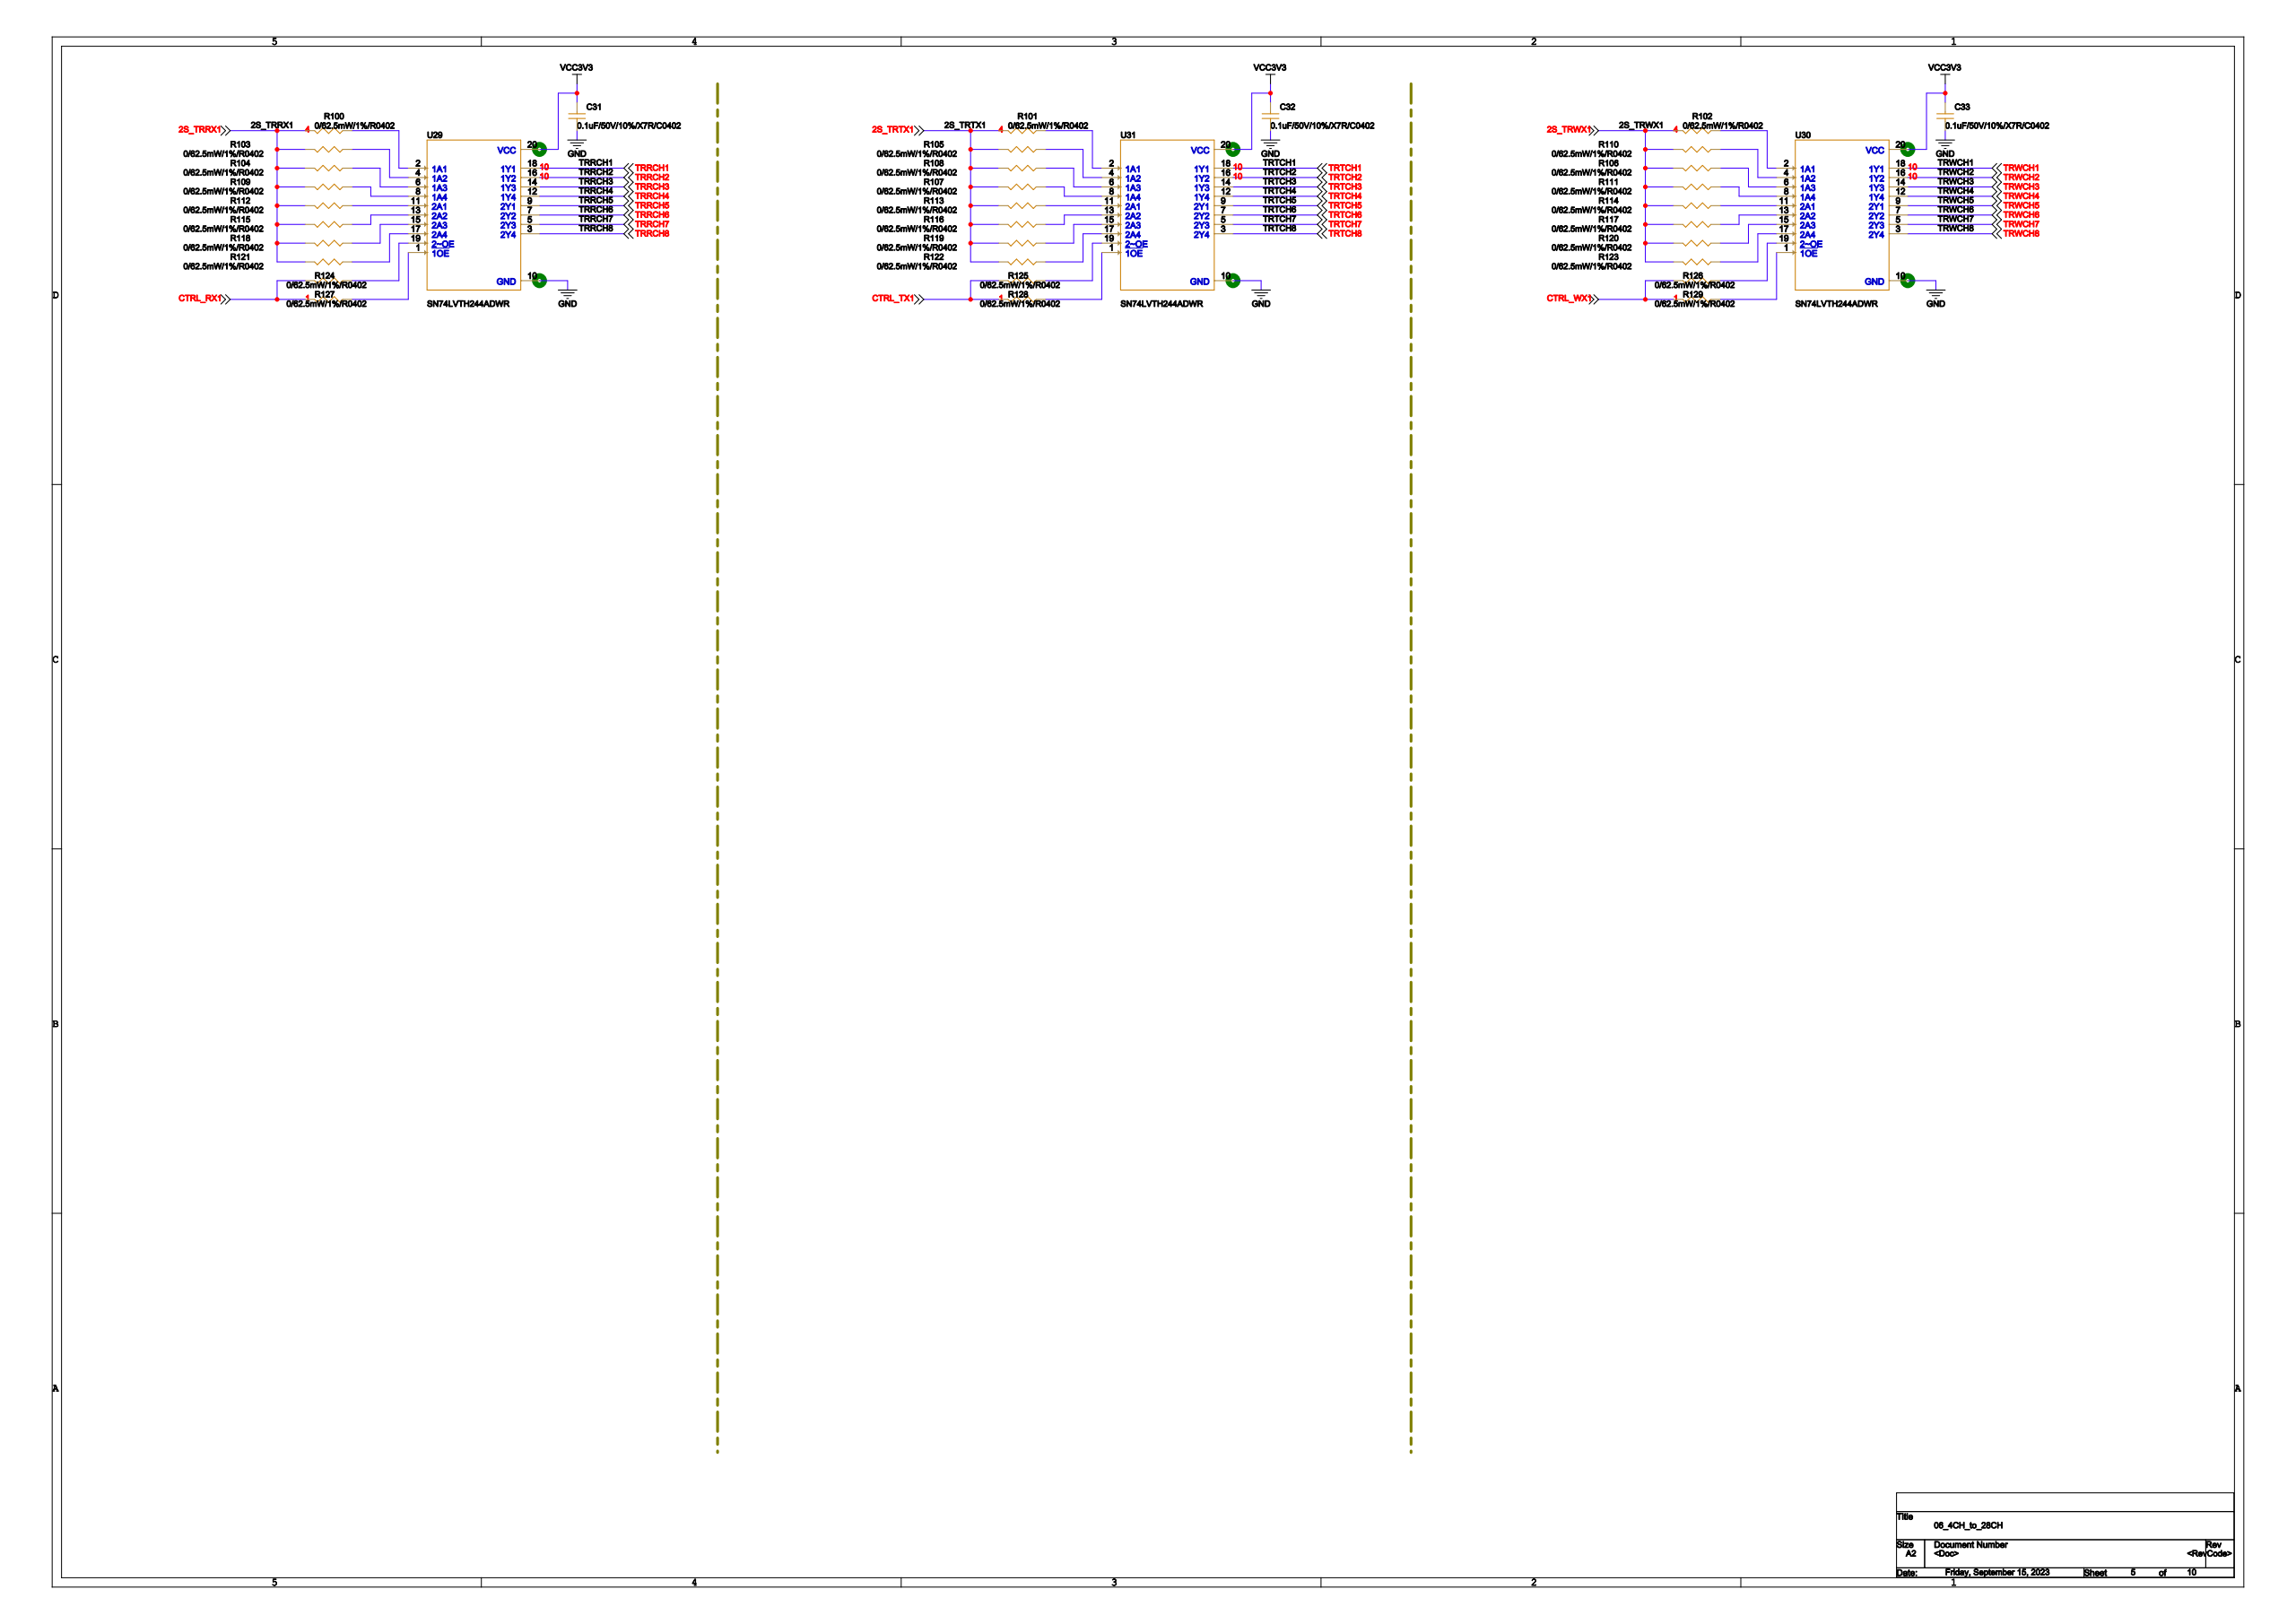Circuit board | Cadence Allegro | 634 parts | 645 nets | one sheet of the schematic
Parts on this sheet (reference | value | footprint):
C31 | 0.1uF/50V/10%/X7R/C0402 | 0402
C32 | 0.1uF/50V/10%/X7R/C0402 | 0402
C33 | 0.1uF/50V/10%/X7R/C0402 | 0402
R100 | 0/62.5mW/1%/R0402 | 0402
R101 | 0/62.5mW/1%/R0402 | 0402
R102 | 0/62.5mW/1%/R0402 | 0402
R103 | 0/62.5mW/1%/R0402 | 0402
R104 | 0/62.5mW/1%/R0402 | 0402
R105 | 0/62.5mW/1%/R0402 | 0402
R106 | 0/62.5mW/1%/R0402 | 0402
R107 | 0/62.5mW/1%/R0402 | 0402
R108 | 0/62.5mW/1%/R0402 | 0402
R109 | 0/62.5mW/1%/R0402 | 0402
R110 | 0/62.5mW/1%/R0402 | 0402
R111 | 0/62.5mW/1%/R0402 | 0402
R112 | 0/62.5mW/1%/R0402 | 0402
R113 | 0/62.5mW/1%/R0402 | 0402
R114 | 0/62.5mW/1%/R0402 | 0402
R115 | 0/62.5mW/1%/R0402 | 0402
R116 | 0/62.5mW/1%/R0402 | 0402
R117 | 0/62.5mW/1%/R0402 | 0402
R118 | 0/62.5mW/1%/R0402 | 0402
R119 | 0/62.5mW/1%/R0402 | 0402
R120 | 0/62.5mW/1%/R0402 | 0402
R121 | 0/62.5mW/1%/R0402 | 0402
R122 | 0/62.5mW/1%/R0402 | 0402
R123 | 0/62.5mW/1%/R0402 | 0402
R124 | 0/62.5mW/1%/R0402 | 0402
R125 | 0/62.5mW/1%/R0402 | 0402
R126 | 0/62.5mW/1%/R0402 | 0402
R127 | 0/62.5mW/1%/R0402 | 0402
R128 | 0/62.5mW/1%/R0402 | 0402
R129 | 0/62.5mW/1%/R0402 | 0402
U29 | SN74LVTH244ADWR | SOIC127P1030X265-20N
U30 | SN74LVTH244ADWR | SOIC127P1030X265-20N
U31 | SN74LVTH244ADWR | SOIC127P1030X265-20N
Nets of these parts (net: part-pin ...):
AGND: C31-2 C32-2 C33-2 U29-10 U30-10 U31-10
3.3V: C31-1 C32-1 C33-1 U29-20 U30-20 U31-20
CTRL_WX1: R126-1 R129-1
CTRL_RX1: R124-1 R127-1
CTRL_TX1: R125-1 R128-1
2S_TRRX1: R100-1 R103-1 R104-1 R109-1 R112-1 R115-1 R118-1 R121-1
N23955636: R100-2 U29-2
2S_TRTX1: R101-1 R105-1 R107-1 R108-1 R113-1 R116-1 R119-1 R122-1
N23963258: R101-2 U31-2
2S_TRWX1: R102-1 R106-1 R110-1 R111-1 R114-1 R117-1 R120-1 R123-1
N23976669: R102-2 U30-2
N23955843: R103-2 U29-4
N23955864: R104-2 U29-6
N23963345: R105-2 U31-4
N23976792: R106-2 U30-6
N23963361: R107-2 U31-8
N23963355: R108-2 U31-6
N23955873: R109-2 U29-8
N23976782: R110-2 U30-4
N23976798: R111-2 U30-8
N23955883: R112-2 U29-11
N23963367: R113-2 U31-11
N23976804: R114-2 U30-11
N23955886: R115-2 U29-13
N23963369: R116-2 U31-13
N23976806: R117-2 U30-13
N23955895: R118-2 U29-15
N23963375: R119-2 U31-15
N23976812: R120-2 U30-15
N23955904: R121-2 U29-17
N23963381: R122-2 U31-17
N23976818: R123-2 U30-17
N23955981: R124-2 U29-19
N23963403: R125-2 U31-19
N23976840: R126-2 U30-19
N23955993: R127-2 U29-1
N23963409: R128-2 U31-1
N23976846: R129-2 U30-1
TRWCH1: U30-18
TRRCH1: U29-18
TRTCH1: U31-18
TRRCH2: U29-16
TRTCH2: U31-16
TRWCH2: U30-16
TRRCH3: U29-14
TRRCH4: U29-12
TRRCH5: U29-9
TRRCH6: U29-7
TRRCH7: U29-5
TRRCH8: U29-3
TRWCH3: U30-14
TRWCH4: U30-12
TRWCH5: U30-9
TRWCH6: U30-7
TRWCH7: U30-5
TRWCH8: U30-3
TRTCH3: U31-14
TRTCH4: U31-12
TRTCH5: U31-9
TRTCH6: U31-7
TRTCH7: U31-5
TRTCH8: U31-3